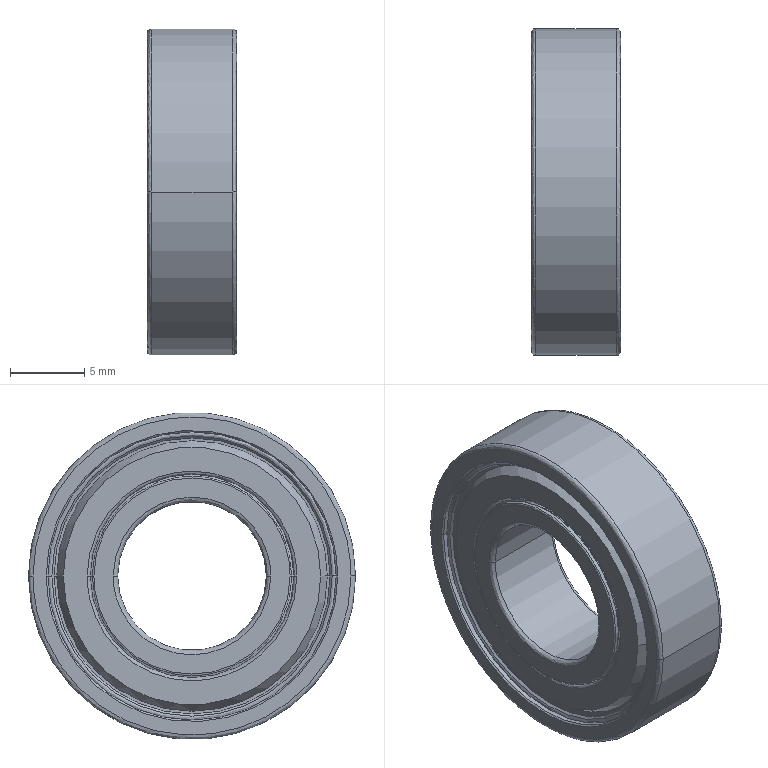Part | SolidWorks | features BaseBody 1 | 1 solid | 136 faces | box 6 x 22 x 22 mm | volume 1447 mm3 | spline 52 | cone 40 | cylinder 32 | plane 12 | commonest cylinder face diameters 12.7 x4 13.4 x4 13.7 x4 14 x4 14.1 x4 18 x4